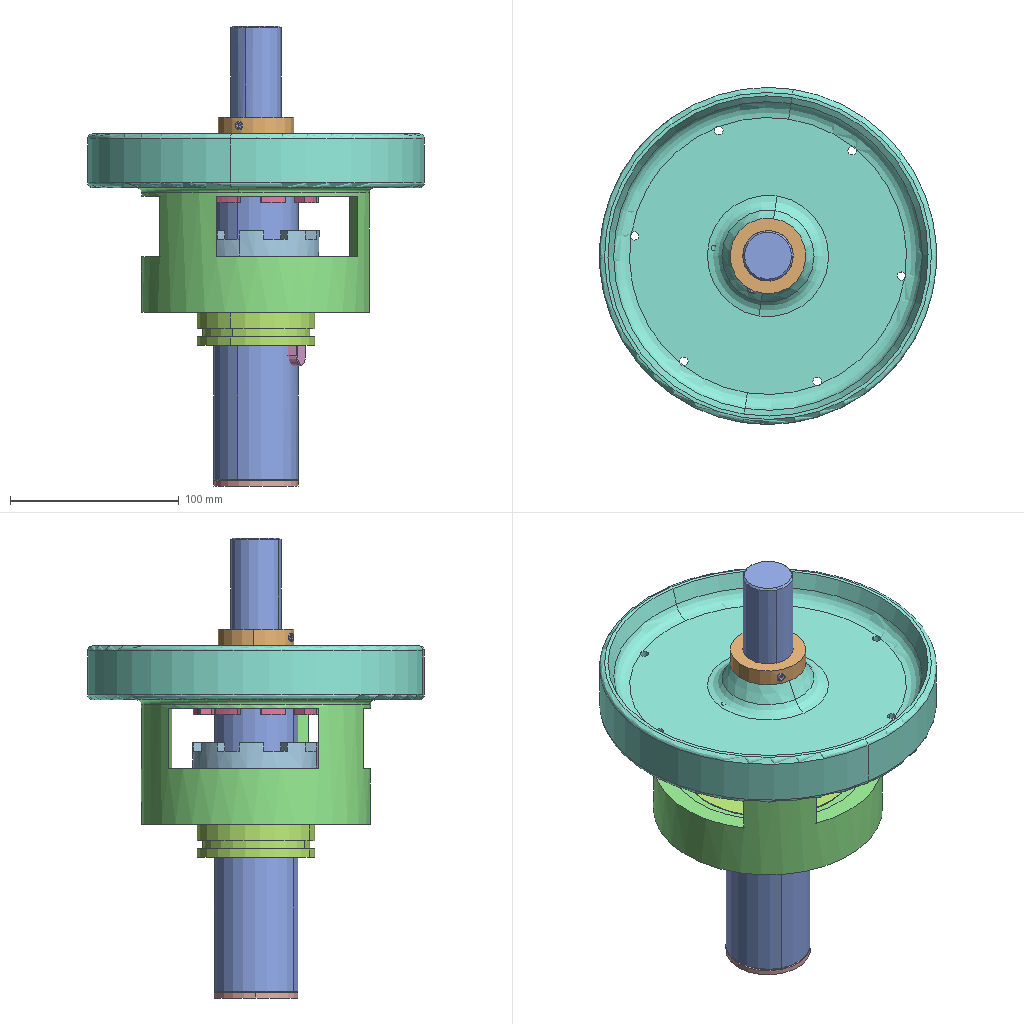Assembly | SolidWorks | 10 different items | 10 placed | box 200 x 200 x 273 mm
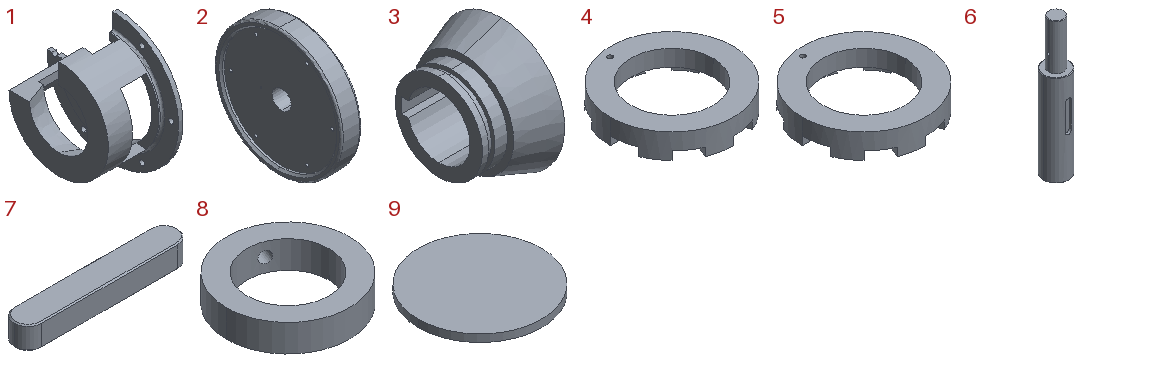Parts list (item | name | quantity | size | volume | features):
1 | - | x1 | 80 x 180 x 180 mm | 298763 mm3 | features ICE 3, CirPattern 1, Fillet 1, Revolution 1
2 | - | x1 | 32 x 200 x 200 mm | 440952 mm3 | features Fillet 2, 3DProfileFeature 1, Chamfer 1, CirPattern 1, HoleWzd 1, ICE 1, Revolution 1
3 | - | x1 | 53 x 101.838 x 101.838 mm | 175302 mm3 | features ICE 2, Revolution 1
4 | - | x1 | 75 x 75 x 15 mm | 28449 mm3 | features ICE 3, Extrusion 1
5 | - | x1 | 75 x 75 x 15 mm | 28449 mm3 | features ICE 3, Extrusion 1
6 | - | x1 | 50 x 50 x 270 mm | 413348 mm3 | features ICE 3, Chamfer 1, Extrusion 1
7 | - | x1 | 72 x 12 x 10 mm | 8292 mm3 | features Chamfer 1, Extrusion 1
8 | - | x1 | 45 x 45 x 10 mm | 8732 mm3 | features 3DProfileFeature 1, Extrusion 1, HoleWzd 1
9 | - | x1 | 50 x 50 x 3 mm | 5890 mm3 | features Extrusion 1
10 | hex socket set screws with cone point gb | x1 | - | - | -
Mates (type | each side: item.copy, entity, surface, feature):
Concentric | 9.1 face cylinder Boss-Extrude1 | 6.1 face cylinder Boss-Extrude1
Coincident | 9.1 face plane Boss-Extrude1 | 6.1 face plane Boss-Extrude1
Concentric | 6.1 face cylinder Boss-Extrude1 | 3.1 face cylinder Revolve1
Coincident | 6.1 face plane Cut-Extrude1 | 3.1 face plane Cut-Extrude1
Coincident | 6.1 face plane Cut-Extrude1 | 7.1 face plane Boss-Extrude1 | 2 times
Concentric | 6.1 face cylinder Cut-Extrude1 | 7.1 face cylinder Boss-Extrude1
Concentric | 6.1 face cylinder Boss-Extrude2 | 2.1 face cylinder Revolve1
Coincident | 6.1 face plane Boss-Extrude1 | 2.1 face plane Revolve1
Concentric | 6.1 face cylinder Boss-Extrude2 | 8.1 face cylinder Boss-Extrude1
Concentric | 6.1 face cylinder Cut-Extrude2 | 8.1 face cylinder M5 Tapped Hole1
Concentric | 6.1 face cylinder Boss-Extrude1 | 1.1 face cone Revolve1
Concentric | 2.1 face cylinder CirPattern1 | 1.1 face cylinder Cut-Extrude1
Coincident | 2.1 face plane Revolve1 | 1.1 face plane Revolve1
Coincident | 3.1 face plane Revolve1 | 4.1 face plane Boss-Extrude1
Concentric | 6.1 face cylinder Boss-Extrude1 | 4.1 face cylinder Boss-Extrude1
Coincident | 2.1 face plane Revolve1 | 5.1 face plane Boss-Extrude1
Concentric | 6.1 face cylinder Boss-Extrude1 | 5.1 face cylinder Boss-Extrude1
Concentric | 3.1 face cylinder Cut-Extrude2 | 4.1 face cylinder Cut-Extrude3
Concentric | 2.1 face cylinder Cut-Extrude1 | 5.1 face cylinder Cut-Extrude3